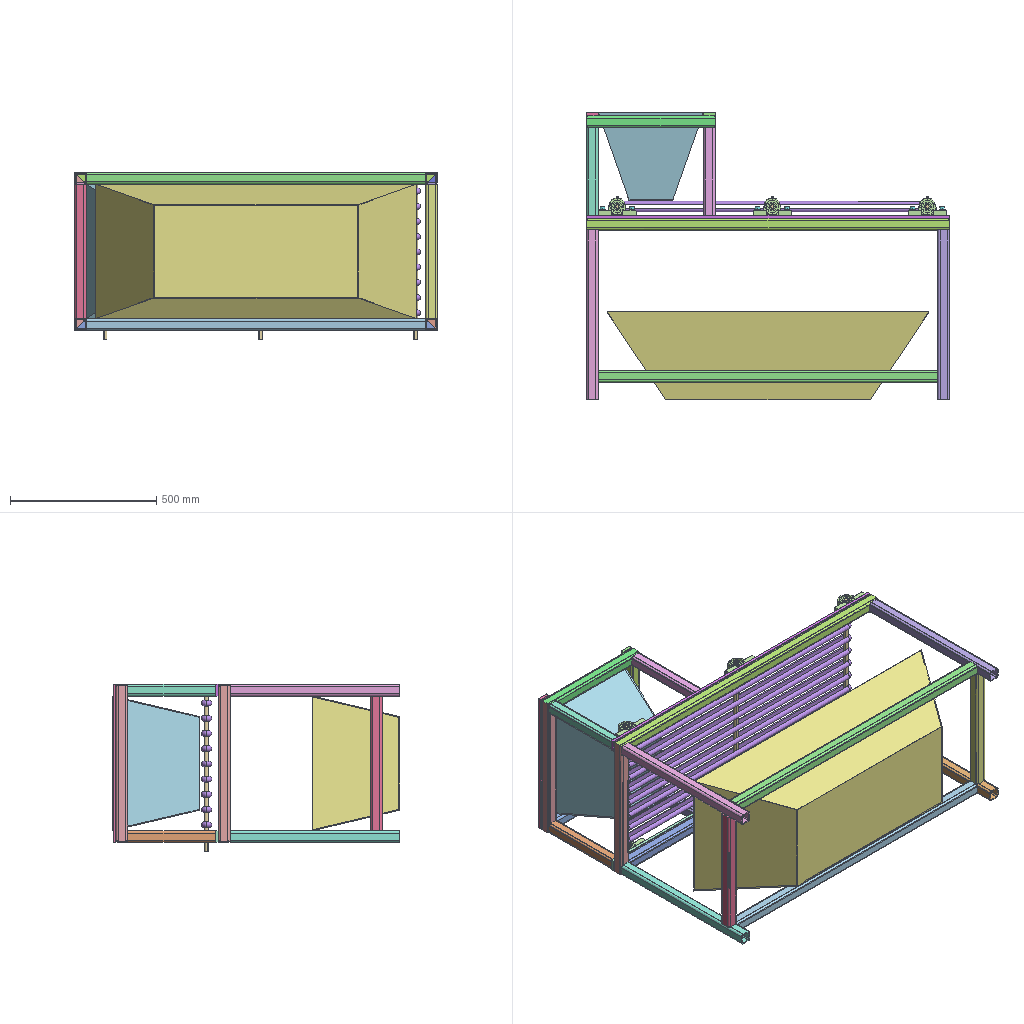Assembly | SolidWorks | 9 different items | 46 placed | box 1240 x 983 x 572 mm
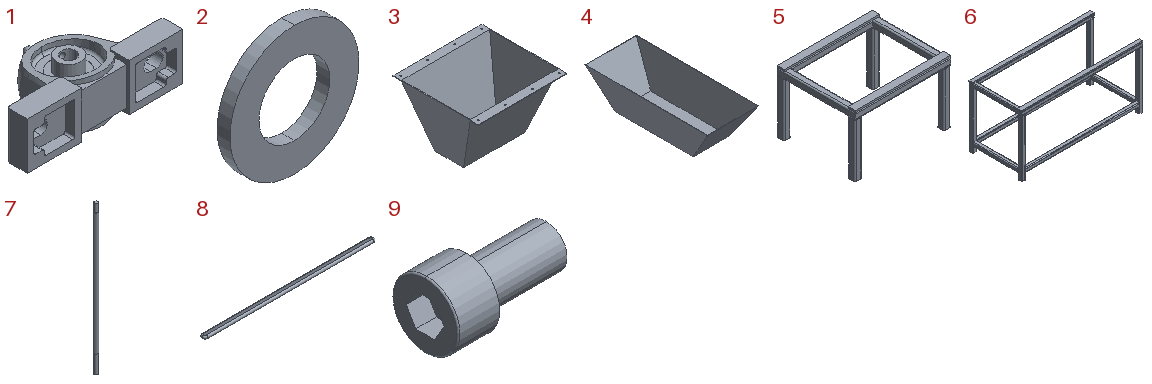Parts list (item | quantity | size | volume | features):
1 | x6 | 129 x 66.06 x 39.46 mm | 93856 mm3 | features Revolution 5, Cut 3, Boss 2, CirPattern 2, ICE 2, RevCut 2, Extrusion 1, RefAxis 1, SweepCut 1
2 | x12 | 20 x 2 x 20 mm | 438.252 mm3 | features Revolution 1
3 | x1 | 460 x 440 x 300 mm | 1312965 mm3 | features ICE 7, Extrusion 1, HoleWzd 1, LPattern 1, MirrorPattern 1, Shell 1
4 | x1 | 460 x 1100 x 300 mm | 3149502 mm3 | features ICE 2, Extrusion 1, Shell 1
5 | x1 | 540 x 440 x 350 mm | 2036389 mm3 | features 3DProfileFeature 1, ICE 1, MirrorSolid 1, WeldMemberFeat 1, WeldmentFeature 1
6 | x1 | 1240 x 540 x 630 mm | 5537770 mm3 | features ICE 2, 3DProfileFeature 1, MirrorSolid 1, WeldMemberFeat 1, WeldmentFeature 1
7 | x3 | 16 x 16 x 563.4 mm | 104482 mm3 | features ICE 2, Extrusion 1
8 | x9 | 1096 x 36 x 20 mm | 345093 mm3 | features Sweep 1
9 | x12 | 30 x 16 x 16 mm | 3295 mm3 | features BlendCut 1, Cut 1, Fillet 1, LPattern 1, RevCut 1, Revolution 1
Mates (type | each side: item.copy, entity, surface, feature):
Parallel | 6.1 face plane Structural Member1 | assembly plane
Width | 6.1 face plane Structural Member1 | 6.1 face plane Structural Member1 | 1.1 face plane Boss-Extrude1 | 1.1 face plane Boss-Extrude1
Coincident | 6.1 face plane Mirror1 | 1.1 face plane Boss-Extrude1
Coincident | 1.1 face plane Boss-Extrude1 | 2.1 face plane Base-Revolve
Concentric | 1.1 face cylinder Cut-Extrude3 | 2.1 face cylinder Base-Revolve
Coincident | 2.1 face plane Base-Revolve | 9.1 face plane Base-Revolve
Concentric | 2.1 face cylinder Base-Revolve | 9.1 face cylinder Base-Revolve
Concentric | 1.1 face cylinder Boss-Revolve5 | 7.1 face cylinder Boss-Extrude1
Coincident | 1.1 face plane Boss-Revolve5 | 7.1 face plane Boss-Extrude1
Concentric | 7.2 face cylinder Boss-Extrude1 | 8.1 edge
Concentric | 7.1 face cylinder Boss-Extrude1 | 8.1 edge
DistanceDim | 6.1 face plane Mirror1 | 8.1 edge
DistanceDim | 6.1 face plane Boss-Extrude1 | 1.2 face plane Boss-Extrude1
Coincident | 6.1 face plane Boss-Extrude1 | 5.1 face plane Structural Member1 | 3 times
Coincident | 5.1 face plane Mirror1 | 3.1 face plane Boss-Extrude4
Coincident | 5.1 face plane Mirror1 | 3.1 face plane Boss-Extrude2
Coincident | 5.1 face plane Structural Member1 | 3.1 face plane Boss-Extrude2
Coincident | 6.1 face plane Structural Member1 | 4.1 face plane Boss-Extrude1
Coincident | 6.1 plane | 4.1 plane | 2 times